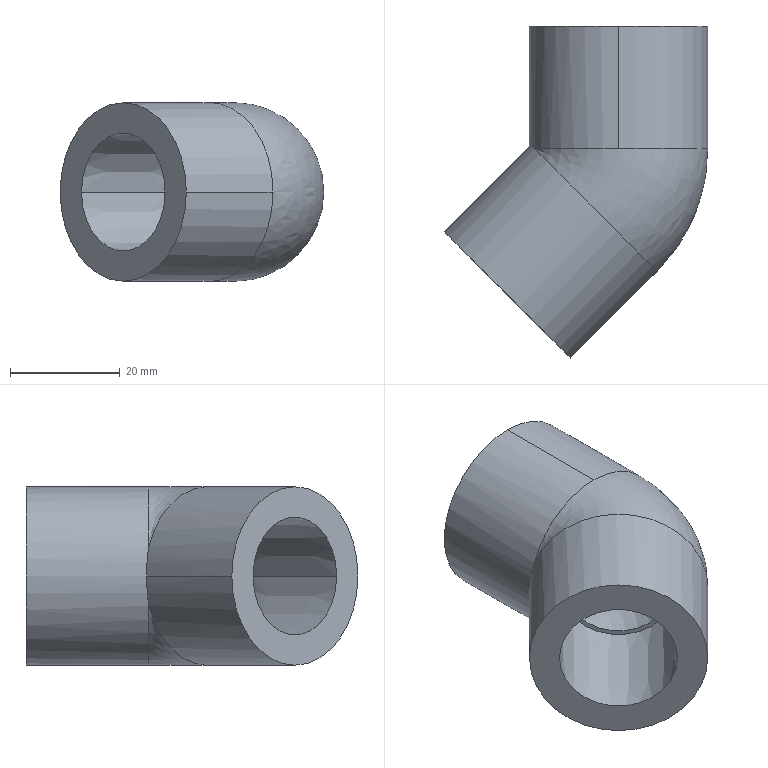Part | SolidWorks | features BaseBody 1 | 1 solid | 15 faces | box 48.046 x 60.492 x 32.512 mm | volume 27507 mm3 | plane 4 | cone 4 | cylinder 4 | torus 2 | spline 1 | commonest cylinder face diameters 32.512 x4
STEP:
#1=CARTESIAN_POINT('',(0.,28.702,10.77));
#2=VERTEX_POINT('',#1);
#3=CARTESIAN_POINT('',(0.,28.702,-10.77));
#4=VERTEX_POINT('',#3);
#5=CARTESIAN_POINT('',(0.,28.702,0.));
#6=DIRECTION('',(0.,1.,0.));
#7=DIRECTION('',(0.,0.,1.));
#8=AXIS2_PLACEMENT_3D('',#5,#6,#7);
#9=CIRCLE('',#8,10.77);
#10=EDGE_CURVE('',#2,#4,#9,.T.);
#11=ORIENTED_EDGE('',*,*,#10,.F.);
#12=CARTESIAN_POINT('',(0.,28.702,0.));
#13=DIRECTION('',(0.,1.,0.));
#14=DIRECTION('',(0.,0.,-1.));
#15=AXIS2_PLACEMENT_3D('',#12,#13,#14);
#16=CIRCLE('',#15,10.77);
#17=EDGE_CURVE('',#4,#2,#16,.T.);
#18=ORIENTED_EDGE('',*,*,#17,.F.);
#19=EDGE_LOOP('',(#11,#18));
#20=FACE_BOUND('',#19,.T.);
#21=CARTESIAN_POINT('',(0.,28.702,-16.256));
#22=VERTEX_POINT('',#21);
#23=CARTESIAN_POINT('',(0.,28.702,16.256));
#24=VERTEX_POINT('',#23);
#25=CARTESIAN_POINT('',(0.,28.702,0.));
#26=DIRECTION('',(0.,-1.,0.));
#27=DIRECTION('',(0.,0.,-1.));
#28=AXIS2_PLACEMENT_3D('',#25,#26,#27);
#29=CIRCLE('',#28,16.256);
#30=EDGE_CURVE('',#22,#24,#29,.T.);
#31=ORIENTED_EDGE('',*,*,#30,.F.);
#32=CARTESIAN_POINT('',(0.,28.702,0.));
#33=DIRECTION('',(0.,-1.,0.));
#34=DIRECTION('',(0.,0.,1.));
#35=AXIS2_PLACEMENT_3D('',#32,#33,#34);
#36=CIRCLE('',#35,16.256);
#37=EDGE_CURVE('',#24,#22,#36,.T.);
#38=ORIENTED_EDGE('',*,*,#37,.F.);
#39=EDGE_LOOP('',(#31,#38));
#40=FACE_OUTER_BOUND('',#39,.T.);
#41=CARTESIAN_POINT('',(16.256,28.702,0.));
#42=DIRECTION('',(0.,1.,0.));
#43=DIRECTION('',(1.,0.,0.));
#44=AXIS2_PLACEMENT_3D('',#41,#42,#43);
#45=PLANE('',#44);
#46=ADVANCED_FACE('',(#20,#40),#45,.T.);
#47=CARTESIAN_POINT('',(9.804,6.35,0.));
#48=VERTEX_POINT('',#47);
#49=CARTESIAN_POINT('',(-9.804,6.35,0.));
#50=VERTEX_POINT('',#49);
#51=CARTESIAN_POINT('',(0.,6.35,0.));
#52=DIRECTION('',(0.,1.,0.));
#53=DIRECTION('',(1.,0.,0.));
#54=AXIS2_PLACEMENT_3D('',#51,#52,#53);
#55=CIRCLE('',#54,9.804);
#56=EDGE_CURVE('',#48,#50,#55,.T.);
#57=ORIENTED_EDGE('',*,*,#56,.F.);
#58=CARTESIAN_POINT('',(0.,6.35,0.));
#59=DIRECTION('',(0.,1.,0.));
#60=DIRECTION('',(-1.,0.,0.));
#61=AXIS2_PLACEMENT_3D('',#58,#59,#60);
#62=CIRCLE('',#61,9.804);
#63=EDGE_CURVE('',#50,#48,#62,.T.);
#64=ORIENTED_EDGE('',*,*,#63,.F.);
#65=EDGE_LOOP('',(#57,#64));
#66=FACE_BOUND('',#65,.T.);
#67=CARTESIAN_POINT('',(0.,6.35,10.617));
#68=VERTEX_POINT('',#67);
#69=CARTESIAN_POINT('',(0.,6.35,-10.617));
#70=VERTEX_POINT('',#69);
#71=CARTESIAN_POINT('',(0.,6.35,0.));
#72=DIRECTION('',(0.,-1.,0.));
#73=DIRECTION('',(0.,0.,1.));
#74=AXIS2_PLACEMENT_3D('',#71,#72,#73);
#75=CIRCLE('',#74,10.617);
#76=EDGE_CURVE('',#68,#70,#75,.T.);
#77=ORIENTED_EDGE('',*,*,#76,.F.);
#78=CARTESIAN_POINT('',(0.,6.35,0.));
#79=DIRECTION('',(0.,-1.,0.));
#80=DIRECTION('',(0.,0.,-1.));
#81=AXIS2_PLACEMENT_3D('',#78,#79,#80);
#82=CIRCLE('',#81,10.617);
#83=EDGE_CURVE('',#70,#68,#82,.T.);
#84=ORIENTED_EDGE('',*,*,#83,.F.);
#85=EDGE_LOOP('',(#77,#84));
#86=FACE_OUTER_BOUND('',#85,.T.);
#87=CARTESIAN_POINT('',(0.,6.35,0.));
#88=DIRECTION('',(0.,1.,0.));
#89=DIRECTION('',(1.,0.,0.));
#90=AXIS2_PLACEMENT_3D('',#87,#88,#89);
#91=PLANE('',#90);
#92=ADVANCED_FACE('',(#66,#86),#91,.T.);
#93=CARTESIAN_POINT('',(7.005,-15.985,0.));
#94=VERTEX_POINT('',#93);
#95=CARTESIAN_POINT('',(-15.33,6.35,5.407));
#96=VERTEX_POINT('',#95);
#97=CARTESIAN_POINT('',(-4.49,-4.49,0.));
#98=DIRECTION('',(-0.7071,-0.7071,0.));
#99=DIRECTION('',(0.7071,-0.7071,0.));
#100=AXIS2_PLACEMENT_3D('',#97,#98,#99);
#101=CIRCLE('',#100,16.256);
#102=EDGE_CURVE('',#94,#96,#101,.T.);
#103=ORIENTED_EDGE('',*,*,#102,.F.);
#104=CARTESIAN_POINT('',(-15.33,6.35,-5.407));
#105=VERTEX_POINT('',#104);
#106=CARTESIAN_POINT('',(-4.49,-4.49,0.));
#107=DIRECTION('',(-0.7071,-0.7071,0.));
#108=DIRECTION('',(-0.6668,0.6668,-0.3326));
#109=AXIS2_PLACEMENT_3D('',#106,#107,#108);
#110=CIRCLE('',#109,16.256);
#111=EDGE_CURVE('',#105,#94,#110,.T.);
#112=ORIENTED_EDGE('',*,*,#111,.F.);
#113=CARTESIAN_POINT('',(0.,6.35,-16.256));
#114=VERTEX_POINT('',#113);
#115=CARTESIAN_POINT('',(0.,6.35,0.));
#116=DIRECTION('',(0.,1.,0.));
#117=DIRECTION('',(0.,0.,-1.));
#118=AXIS2_PLACEMENT_3D('',#115,#116,#117);
#119=CIRCLE('',#118,16.256);
#120=EDGE_CURVE('',#114,#105,#119,.T.);
#121=ORIENTED_EDGE('',*,*,#120,.F.);
#122=CARTESIAN_POINT('',(0.,6.35,16.256));
#123=VERTEX_POINT('',#122);
#124=CARTESIAN_POINT('',(0.,6.35,0.));
#125=DIRECTION('',(0.,1.,0.));
#126=DIRECTION('',(0.,0.,1.));
#127=AXIS2_PLACEMENT_3D('',#124,#125,#126);
#128=CIRCLE('',#127,16.256);
#129=EDGE_CURVE('',#123,#114,#128,.T.);
#130=ORIENTED_EDGE('',*,*,#129,.F.);
#131=CARTESIAN_POINT('',(0.,6.35,0.));
#132=DIRECTION('',(0.,1.,0.));
#133=DIRECTION('',(-0.9431,0.,0.3326));
#134=AXIS2_PLACEMENT_3D('',#131,#132,#133);
#135=CIRCLE('',#134,16.256);
#136=EDGE_CURVE('',#96,#123,#135,.T.);
#137=ORIENTED_EDGE('',*,*,#136,.F.);
#138=EDGE_LOOP('',(#103,#112,#121,#130,#137));
#139=FACE_OUTER_BOUND('',#138,.T.);
#140=CARTESIAN_POINT('',(-15.33,6.35,5.407));
#141=CARTESIAN_POINT('',(-15.33,6.35,5.407));
#142=CARTESIAN_POINT('',(-15.33,6.35,5.407));
#143=CARTESIAN_POINT('',(-12.106,3.125,18.336));
#144=CARTESIAN_POINT('',(-10.77,4.461,18.336));
#145=CARTESIAN_POINT('',(-10.77,6.35,18.336));
#146=CARTESIAN_POINT('',(-2.55,-6.43,16.023));
#147=CARTESIAN_POINT('',(2.743,-1.136,16.023));
#148=CARTESIAN_POINT('',(2.743,6.35,16.023));
#149=CARTESIAN_POINT('',(7.005,-15.985,13.71));
#150=CARTESIAN_POINT('',(16.256,-6.733,13.71));
#151=CARTESIAN_POINT('',(16.256,6.35,13.71));
#152=CARTESIAN_POINT('',(7.005,-15.985,0.));
#153=CARTESIAN_POINT('',(16.256,-6.733,0.));
#154=CARTESIAN_POINT('',(16.256,6.35,0.));
#155=CARTESIAN_POINT('',(7.005,-15.985,-13.71));
#156=CARTESIAN_POINT('',(16.256,-6.733,-13.71));
#157=CARTESIAN_POINT('',(16.256,6.35,-13.71));
#158=CARTESIAN_POINT('',(-2.55,-6.43,-16.023));
#159=CARTESIAN_POINT('',(2.743,-1.136,-16.023));
#160=CARTESIAN_POINT('',(2.743,6.35,-16.023));
#161=CARTESIAN_POINT('',(-12.106,3.125,-18.336));
#162=CARTESIAN_POINT('',(-10.77,4.461,-18.336));
#163=CARTESIAN_POINT('',(-10.77,6.35,-18.336));
#164=CARTESIAN_POINT('',(-15.33,6.35,-5.407));
#165=CARTESIAN_POINT('',(-15.33,6.35,-5.407));
#166=CARTESIAN_POINT('',(-15.33,6.35,-5.407));
#167=(BOUNDED_SURFACE()B_SPLINE_SURFACE(2,2,((#140,#141,#142),(#143,#144,#145),(#146,#147,#148),(#149,#150,#151),(#152,#153,#154),(#155,#156,#157),(#158,#159,#160),(#161,#162,#163),(#164,#165,#166)),.UNSPECIFIED.,.F.,.F.,.F.)B_SPLINE_SURFACE_WITH_KNOTS((3,2,2,2,3),(3,3),(-2.802,-1.401,0.,1.401,2.802),(-3.142,-2.356),.UNSPECIFIED.)GEOMETRIC_REPRESENTATION_ITEM()RATIONAL_B_SPLINE_SURFACE(((1.,0.9239,1.),(0.7644,0.7063,0.7644),(1.,0.9239,1.),(0.7644,0.7063,0.7644),(1.,0.9239,1.),(0.7644,0.7063,0.7644),(1.,0.9239,1.),(0.7644,0.7063,0.7644),(1.,0.9239,1.)))REPRESENTATION_ITEM('')SURFACE());
#168=ADVANCED_FACE('',(#139),#167,.T.);
#169=CARTESIAN_POINT('',(2.443,-11.423,0.));
#170=VERTEX_POINT('',#169);
#171=CARTESIAN_POINT('',(-11.423,2.443,0.));
#172=VERTEX_POINT('',#171);
#173=CARTESIAN_POINT('',(-4.49,-4.49,0.));
#174=DIRECTION('',(-0.7071,-0.7071,0.));
#175=DIRECTION('',(0.7071,-0.7071,0.));
#176=AXIS2_PLACEMENT_3D('',#173,#174,#175);
#177=CIRCLE('',#176,9.804);
#178=EDGE_CURVE('',#170,#172,#177,.T.);
#179=ORIENTED_EDGE('',*,*,#178,.F.);
#180=CARTESIAN_POINT('',(-4.49,-4.49,0.));
#181=DIRECTION('',(-0.7071,-0.7071,0.));
#182=DIRECTION('',(-0.7071,0.7071,0.));
#183=AXIS2_PLACEMENT_3D('',#180,#181,#182);
#184=CIRCLE('',#183,9.804);
#185=EDGE_CURVE('',#172,#170,#184,.T.);
#186=ORIENTED_EDGE('',*,*,#185,.F.);
#187=EDGE_LOOP('',(#179,#186));
#188=FACE_BOUND('',#187,.T.);
#189=CARTESIAN_POINT('',(3.017,-11.998,0.));
#190=VERTEX_POINT('',#189);
#191=CARTESIAN_POINT('',(-11.998,3.017,0.));
#192=VERTEX_POINT('',#191);
#193=CARTESIAN_POINT('',(-4.49,-4.49,0.));
#194=DIRECTION('',(0.7071,0.7071,0.));
#195=DIRECTION('',(0.7071,-0.7071,0.));
#196=AXIS2_PLACEMENT_3D('',#193,#194,#195);
#197=CIRCLE('',#196,10.617);
#198=EDGE_CURVE('',#190,#192,#197,.T.);
#199=ORIENTED_EDGE('',*,*,#198,.F.);
#200=CARTESIAN_POINT('',(-4.49,-4.49,0.));
#201=DIRECTION('',(0.7071,0.7071,0.));
#202=DIRECTION('',(-0.7071,0.7071,0.));
#203=AXIS2_PLACEMENT_3D('',#200,#201,#202);
#204=CIRCLE('',#203,10.617);
#205=EDGE_CURVE('',#192,#190,#204,.T.);
#206=ORIENTED_EDGE('',*,*,#205,.F.);
#207=EDGE_LOOP('',(#199,#206));
#208=FACE_OUTER_BOUND('',#207,.T.);
#209=CARTESIAN_POINT('',(-4.49,-4.49,0.));
#210=DIRECTION('',(-0.7071,-0.7071,0.));
#211=DIRECTION('',(-0.7071,0.7071,0.));
#212=AXIS2_PLACEMENT_3D('',#209,#210,#211);
#213=PLANE('',#212);
#214=ADVANCED_FACE('',(#188,#208),#213,.T.);
#215=CARTESIAN_POINT('',(-12.68,-27.911,0.));
#216=VERTEX_POINT('',#215);
#217=CARTESIAN_POINT('',(-27.911,-12.68,0.));
#218=VERTEX_POINT('',#217);
#219=CARTESIAN_POINT('',(-20.295,-20.295,0.));
#220=DIRECTION('',(-0.7071,-0.7071,0.));
#221=DIRECTION('',(0.7071,-0.7071,0.));
#222=AXIS2_PLACEMENT_3D('',#219,#220,#221);
#223=CIRCLE('',#222,10.77);
#224=EDGE_CURVE('',#216,#218,#223,.T.);
#225=ORIENTED_EDGE('',*,*,#224,.F.);
#226=CARTESIAN_POINT('',(-20.295,-20.295,0.));
#227=DIRECTION('',(-0.7071,-0.7071,0.));
#228=DIRECTION('',(-0.7071,0.7071,0.));
#229=AXIS2_PLACEMENT_3D('',#226,#227,#228);
#230=CIRCLE('',#229,10.77);
#231=EDGE_CURVE('',#218,#216,#230,.T.);
#232=ORIENTED_EDGE('',*,*,#231,.F.);
#233=EDGE_LOOP('',(#225,#232));
#234=FACE_BOUND('',#233,.T.);
#235=CARTESIAN_POINT('',(-8.801,-31.79,0.));
#236=VERTEX_POINT('',#235);
#237=CARTESIAN_POINT('',(-31.79,-8.801,0.));
#238=VERTEX_POINT('',#237);
#239=CARTESIAN_POINT('',(-20.295,-20.295,0.));
#240=DIRECTION('',(0.7071,0.7071,0.));
#241=DIRECTION('',(0.7071,-0.7071,0.));
#242=AXIS2_PLACEMENT_3D('',#239,#240,#241);
#243=CIRCLE('',#242,16.256);
#244=EDGE_CURVE('',#236,#238,#243,.T.);
#245=ORIENTED_EDGE('',*,*,#244,.F.);
#246=CARTESIAN_POINT('',(-20.295,-20.295,0.));
#247=DIRECTION('',(0.7071,0.7071,0.));
#248=DIRECTION('',(-0.7071,0.7071,0.));
#249=AXIS2_PLACEMENT_3D('',#246,#247,#248);
#250=CIRCLE('',#249,16.256);
#251=EDGE_CURVE('',#238,#236,#250,.T.);
#252=ORIENTED_EDGE('',*,*,#251,.F.);
#253=EDGE_LOOP('',(#245,#252));
#254=FACE_OUTER_BOUND('',#253,.T.);
#255=CARTESIAN_POINT('',(-8.801,-31.79,0.));
#256=DIRECTION('',(-0.7071,-0.7071,0.));
#257=DIRECTION('',(-0.7071,0.7071,0.));
#258=AXIS2_PLACEMENT_3D('',#255,#256,#257);
#259=PLANE('',#258);
#260=ADVANCED_FACE('',(#234,#254),#259,.T.);
#261=ORIENTED_EDGE('',*,*,#205,.T.);
#262=CARTESIAN_POINT('',(-12.68,-27.911,0.));
#263=DIRECTION('',(0.7023,0.7119,0.));
#264=VECTOR('',#263,1000.);
#265=LINE('',#262,#264);
#266=EDGE_CURVE('',#216,#190,#265,.T.);
#267=ORIENTED_EDGE('',*,*,#266,.F.);
#268=ORIENTED_EDGE('',*,*,#224,.T.);
#269=CARTESIAN_POINT('',(-11.998,3.017,0.));
#270=DIRECTION('',(-0.7119,-0.7023,0.));
#271=VECTOR('',#270,1000.);
#272=LINE('',#269,#271);
#273=EDGE_CURVE('',#192,#218,#272,.T.);
#274=ORIENTED_EDGE('',*,*,#273,.F.);
#275=EDGE_LOOP('',(#261,#267,#268,#274));
#276=FACE_OUTER_BOUND('',#275,.T.);
#277=CARTESIAN_POINT('',(37.941,37.941,0.));
#278=DIRECTION('',(-0.7071,-0.7071,0.));
#279=DIRECTION('',(0.7071,-0.7071,0.));
#280=AXIS2_PLACEMENT_3D('',#277,#278,#279);
#281=CONICAL_SURFACE('',#280,10.208,0.006818);
#282=ADVANCED_FACE('',(#276),#281,.F.);
#283=ORIENTED_EDGE('',*,*,#273,.T.);
#284=ORIENTED_EDGE('',*,*,#231,.T.);
#285=ORIENTED_EDGE('',*,*,#266,.T.);
#286=ORIENTED_EDGE('',*,*,#198,.T.);
#287=EDGE_LOOP('',(#283,#284,#285,#286));
#288=FACE_OUTER_BOUND('',#287,.T.);
#289=CARTESIAN_POINT('',(37.941,37.941,0.));
#290=DIRECTION('',(-0.7071,-0.7071,0.));
#291=DIRECTION('',(0.7071,-0.7071,0.));
#292=AXIS2_PLACEMENT_3D('',#289,#290,#291);
#293=CONICAL_SURFACE('',#292,10.208,0.006818);
#294=ADVANCED_FACE('',(#288),#293,.F.);
#295=ORIENTED_EDGE('',*,*,#251,.T.);
#296=CARTESIAN_POINT('',(7.005,-15.985,0.));
#297=DIRECTION('',(-0.7071,-0.7071,0.));
#298=VECTOR('',#297,1000.);
#299=LINE('',#296,#298);
#300=EDGE_CURVE('',#94,#236,#299,.T.);
#301=ORIENTED_EDGE('',*,*,#300,.F.);
#302=ORIENTED_EDGE('',*,*,#102,.T.);
#303=CARTESIAN_POINT('',(-16.256,6.733,0.));
#304=VERTEX_POINT('',#303);
#305=CARTESIAN_POINT('',(-16.256,6.733,0.));
#306=CARTESIAN_POINT('',(-16.256,6.733,1.846));
#307=CARTESIAN_POINT('',(-15.944,6.604,3.666));
#308=CARTESIAN_POINT('',(-15.33,6.35,5.407));
#309=(BOUNDED_CURVE()B_SPLINE_CURVE(3,(#305,#306,#307,#308),.UNSPECIFIED.,.F.,.T.)B_SPLINE_CURVE_WITH_KNOTS((4,4),(6.283,6.622),.UNSPECIFIED.)CURVE()GEOMETRIC_REPRESENTATION_ITEM()RATIONAL_B_SPLINE_CURVE((1.,0.9904,0.9904,1.))REPRESENTATION_ITEM(''));
#310=EDGE_CURVE('',#304,#96,#309,.T.);
#311=ORIENTED_EDGE('',*,*,#310,.F.);
#312=CARTESIAN_POINT('',(-31.79,-8.801,0.));
#313=DIRECTION('',(0.7071,0.7071,0.));
#314=VECTOR('',#313,1000.);
#315=LINE('',#312,#314);
#316=EDGE_CURVE('',#238,#304,#315,.T.);
#317=ORIENTED_EDGE('',*,*,#316,.F.);
#318=EDGE_LOOP('',(#295,#301,#302,#311,#317));
#319=FACE_OUTER_BOUND('',#318,.T.);
#320=CARTESIAN_POINT('',(-4.49,-4.49,0.));
#321=DIRECTION('',(-0.7071,-0.7071,0.));
#322=DIRECTION('',(0.7071,-0.7071,0.));
#323=AXIS2_PLACEMENT_3D('',#320,#321,#322);
#324=CYLINDRICAL_SURFACE('',#323,16.256);
#325=ADVANCED_FACE('',(#319),#324,.T.);
#326=ORIENTED_EDGE('',*,*,#316,.T.);
#327=CARTESIAN_POINT('',(-15.33,6.35,-5.407));
#328=CARTESIAN_POINT('',(-15.944,6.604,-3.666));
#329=CARTESIAN_POINT('',(-16.256,6.733,-1.846));
#330=CARTESIAN_POINT('',(-16.256,6.733,0.));
#331=(BOUNDED_CURVE()B_SPLINE_CURVE(3,(#327,#328,#329,#330),.UNSPECIFIED.,.F.,.F.)B_SPLINE_CURVE_WITH_KNOTS((4,4),(5.944,6.283),.UNSPECIFIED.)CURVE()GEOMETRIC_REPRESENTATION_ITEM()RATIONAL_B_SPLINE_CURVE((1.,0.9904,0.9904,1.))REPRESENTATION_ITEM(''));
#332=EDGE_CURVE('',#105,#304,#331,.T.);
#333=ORIENTED_EDGE('',*,*,#332,.F.);
#334=ORIENTED_EDGE('',*,*,#111,.T.);
#335=ORIENTED_EDGE('',*,*,#300,.T.);
#336=ORIENTED_EDGE('',*,*,#244,.T.);
#337=EDGE_LOOP('',(#326,#333,#334,#335,#336));
#338=FACE_OUTER_BOUND('',#337,.T.);
#339=CARTESIAN_POINT('',(-4.49,-4.49,0.));
#340=DIRECTION('',(-0.7071,-0.7071,0.));
#341=DIRECTION('',(0.7071,-0.7071,0.));
#342=AXIS2_PLACEMENT_3D('',#339,#340,#341);
#343=CYLINDRICAL_SURFACE('',#342,16.256);
#344=ADVANCED_FACE('',(#338),#343,.T.);
#345=ORIENTED_EDGE('',*,*,#136,.T.);
#346=CARTESIAN_POINT('',(0.,6.35,16.256));
#347=DIRECTION('',(0.,1.,0.));
#348=VECTOR('',#347,1000.);
#349=LINE('',#346,#348);
#350=EDGE_CURVE('',#123,#24,#349,.T.);
#351=ORIENTED_EDGE('',*,*,#350,.T.);
#352=ORIENTED_EDGE('',*,*,#37,.T.);
#353=CARTESIAN_POINT('',(0.,6.35,-16.256));
#354=DIRECTION('',(0.,1.,0.));
#355=VECTOR('',#354,1000.);
#356=LINE('',#353,#355);
#357=EDGE_CURVE('',#114,#22,#356,.T.);
#358=ORIENTED_EDGE('',*,*,#357,.F.);
#359=ORIENTED_EDGE('',*,*,#120,.T.);
#360=ORIENTED_EDGE('',*,*,#332,.T.);
#361=ORIENTED_EDGE('',*,*,#310,.T.);
#362=EDGE_LOOP('',(#345,#351,#352,#358,#359,#360,#361));
#363=FACE_OUTER_BOUND('',#362,.T.);
#364=CARTESIAN_POINT('',(0.,28.702,0.));
#365=DIRECTION('',(0.,-1.,0.));
#366=DIRECTION('',(0.,0.,-1.));
#367=AXIS2_PLACEMENT_3D('',#364,#365,#366);
#368=CYLINDRICAL_SURFACE('',#367,16.256);
#369=ADVANCED_FACE('',(#363),#368,.T.);
#370=ORIENTED_EDGE('',*,*,#350,.F.);
#371=ORIENTED_EDGE('',*,*,#129,.T.);
#372=ORIENTED_EDGE('',*,*,#357,.T.);
#373=ORIENTED_EDGE('',*,*,#30,.T.);
#374=EDGE_LOOP('',(#370,#371,#372,#373));
#375=FACE_OUTER_BOUND('',#374,.T.);
#376=CARTESIAN_POINT('',(0.,28.702,0.));
#377=DIRECTION('',(0.,-1.,0.));
#378=DIRECTION('',(0.,0.,-1.));
#379=AXIS2_PLACEMENT_3D('',#376,#377,#378);
#380=CYLINDRICAL_SURFACE('',#379,16.256);
#381=ADVANCED_FACE('',(#375),#380,.T.);
#382=ORIENTED_EDGE('',*,*,#83,.T.);
#383=CARTESIAN_POINT('',(0.,28.702,10.77));
#384=DIRECTION('',(0.,-1.,-0.006818));
#385=VECTOR('',#384,1000.);
#386=LINE('',#383,#385);
#387=EDGE_CURVE('',#2,#68,#386,.T.);
#388=ORIENTED_EDGE('',*,*,#387,.F.);
#389=ORIENTED_EDGE('',*,*,#10,.T.);
#390=CARTESIAN_POINT('',(0.,6.35,-10.617));
#391=DIRECTION('',(0.,1.,-0.006818));
#392=VECTOR('',#391,1000.);
#393=LINE('',#390,#392);
#394=EDGE_CURVE('',#70,#4,#393,.T.);
#395=ORIENTED_EDGE('',*,*,#394,.F.);
#396=EDGE_LOOP('',(#382,#388,#389,#395));
#397=FACE_OUTER_BOUND('',#396,.T.);
#398=CARTESIAN_POINT('',(0.,-20.256,0.));
#399=DIRECTION('',(0.,1.,0.));
#400=DIRECTION('',(0.,0.,1.));
#401=AXIS2_PLACEMENT_3D('',#398,#399,#400);
#402=CONICAL_SURFACE('',#401,10.436,0.006818);
#403=ADVANCED_FACE('',(#397),#402,.F.);
#404=ORIENTED_EDGE('',*,*,#394,.T.);
#405=ORIENTED_EDGE('',*,*,#17,.T.);
#406=ORIENTED_EDGE('',*,*,#387,.T.);
#407=ORIENTED_EDGE('',*,*,#76,.T.);
#408=EDGE_LOOP('',(#404,#405,#406,#407));
#409=FACE_OUTER_BOUND('',#408,.T.);
#410=CARTESIAN_POINT('',(0.,-20.256,0.));
#411=DIRECTION('',(0.,1.,0.));
#412=DIRECTION('',(0.,0.,1.));
#413=AXIS2_PLACEMENT_3D('',#410,#411,#412);
#414=CONICAL_SURFACE('',#413,10.436,0.006818);
#415=ADVANCED_FACE('',(#409),#414,.F.);
#416=ORIENTED_EDGE('',*,*,#63,.T.);
#417=CARTESIAN_POINT('',(-15.33,6.35,0.));
#418=DIRECTION('',(0.,0.,1.));
#419=DIRECTION('',(0.7071,-0.7071,0.));
#420=AXIS2_PLACEMENT_3D('',#417,#418,#419);
#421=CIRCLE('',#420,25.135);
#422=EDGE_CURVE('',#170,#48,#421,.T.);
#423=ORIENTED_EDGE('',*,*,#422,.F.);
#424=ORIENTED_EDGE('',*,*,#178,.T.);
#425=CARTESIAN_POINT('',(-15.33,6.35,0.));
#426=DIRECTION('',(0.,0.,-1.));
#427=DIRECTION('',(1.,0.,0.));
#428=AXIS2_PLACEMENT_3D('',#425,#426,#427);
#429=CIRCLE('',#428,5.526);
#430=EDGE_CURVE('',#50,#172,#429,.T.);
#431=ORIENTED_EDGE('',*,*,#430,.F.);
#432=EDGE_LOOP('',(#416,#423,#424,#431));
#433=FACE_OUTER_BOUND('',#432,.T.);
#434=CARTESIAN_POINT('',(-15.33,6.35,0.));
#435=DIRECTION('',(0.,0.,-1.));
#436=DIRECTION('',(0.7071,-0.7071,0.));
#437=AXIS2_PLACEMENT_3D('',#434,#435,#436);
#438=TOROIDAL_SURFACE('',#437,15.33,9.804);
#439=ADVANCED_FACE('',(#433),#438,.F.);
#440=ORIENTED_EDGE('',*,*,#430,.T.);
#441=ORIENTED_EDGE('',*,*,#185,.T.);
#442=ORIENTED_EDGE('',*,*,#422,.T.);
#443=ORIENTED_EDGE('',*,*,#56,.T.);
#444=EDGE_LOOP('',(#440,#441,#442,#443));
#445=FACE_OUTER_BOUND('',#444,.T.);
#446=CARTESIAN_POINT('',(-15.33,6.35,0.));
#447=DIRECTION('',(0.,0.,-1.));
#448=DIRECTION('',(0.7071,-0.7071,0.));
#449=AXIS2_PLACEMENT_3D('',#446,#447,#448);
#450=TOROIDAL_SURFACE('',#449,15.33,9.804);
#451=ADVANCED_FACE('',(#445),#450,.F.);
#452=CLOSED_SHELL('',(#46,#92,#168,#214,#260,#282,#294,#325,#344,#369,#381,#403,#415,#439,#451));
#453=MANIFOLD_SOLID_BREP('',#452);
#454=CARTESIAN_POINT('',(0.,0.,0.));
#455=DIRECTION('',(0.,0.,1.));
#456=DIRECTION('',(1.,0.,0.));
#457=AXIS2_PLACEMENT_3D('',#454,#455,#456);
#458=(LENGTH_UNIT()NAMED_UNIT(*)SI_UNIT(.MILLI.,.METRE.));
#459=UNCERTAINTY_MEASURE_WITH_UNIT(LENGTH_MEASURE(0.00001),#458,'','');
#460=(NAMED_UNIT(*)PLANE_ANGLE_UNIT()SI_UNIT($,.RADIAN.));
#461=(NAMED_UNIT(*)SI_UNIT($,.STERADIAN.)SOLID_ANGLE_UNIT());
#462=(GEOMETRIC_REPRESENTATION_CONTEXT(3)GLOBAL_UNCERTAINTY_ASSIGNED_CONTEXT((#459))GLOBAL_UNIT_ASSIGNED_CONTEXT((#458,#460,#461))REPRESENTATION_CONTEXT('',''));
#463=ADVANCED_BREP_SHAPE_REPRESENTATION('',(#453,#457),#462);